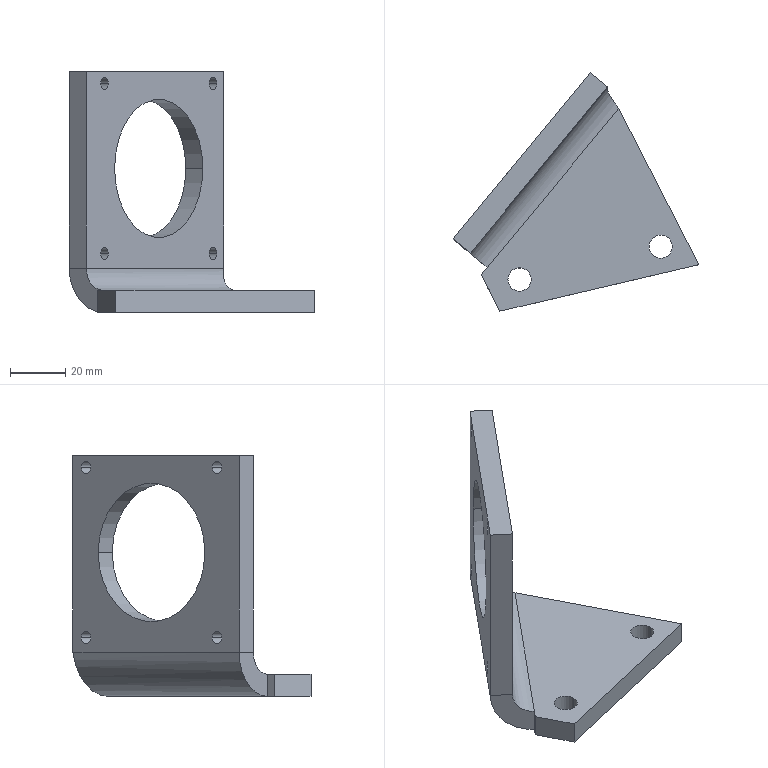Part | SolidWorks | features Cut 2, ICE 2, RefAxis 2, EdgeFlange 1, FlatPattern 1, SMBaseFlange 1, SheetMetal 1 | 1 solid | 29 faces | box 88.743 x 86.001 x 87 mm | volume 61033 mm3 | cylinder 16 | plane 12 | spline 1 | commonest cylinder face diameters 4.4 x8 8.382 x2 8.4 x2 50 x2 16 x1 32 x1
STEP:
#1=CARTESIAN_POINT('',(-8.739,128.402,52.));
#2=VERTEX_POINT('',#1);
#3=CARTESIAN_POINT('',(23.129,166.93,52.));
#4=VERTEX_POINT('',#3);
#5=CARTESIAN_POINT('',(7.195,147.666,52.));
#6=DIRECTION('',(0.7706,-0.6374,0.));
#7=DIRECTION('',(0.6374,0.7706,0.));
#8=AXIS2_PLACEMENT_3D('',#5,#6,#7);
#9=CIRCLE('',#8,25.);
#10=EDGE_CURVE('',#2,#4,#9,.T.);
#11=ORIENTED_EDGE('',*,*,#10,.F.);
#12=CARTESIAN_POINT('',(-2.574,123.303,52.));
#13=VERTEX_POINT('',#12);
#14=CARTESIAN_POINT('',(-10.28,129.677,52.));
#15=DIRECTION('',(0.7706,-0.6374,0.));
#16=VECTOR('',#15,1000.);
#17=LINE('',#14,#16);
#18=EDGE_CURVE('',#2,#13,#17,.T.);
#19=ORIENTED_EDGE('',*,*,#18,.T.);
#20=CARTESIAN_POINT('',(29.293,161.832,52.));
#21=VERTEX_POINT('',#20);
#22=CARTESIAN_POINT('',(13.36,142.567,52.));
#23=DIRECTION('',(0.7706,-0.6374,0.));
#24=DIRECTION('',(0.6374,0.7706,0.));
#25=AXIS2_PLACEMENT_3D('',#22,#23,#24);
#26=CIRCLE('',#25,25.);
#27=EDGE_CURVE('',#13,#21,#26,.T.);
#28=ORIENTED_EDGE('',*,*,#27,.T.);
#29=CARTESIAN_POINT('',(21.588,168.205,52.));
#30=DIRECTION('',(0.7706,-0.6374,0.));
#31=VECTOR('',#30,1000.);
#32=LINE('',#29,#31);
#33=EDGE_CURVE('',#4,#21,#32,.T.);
#34=ORIENTED_EDGE('',*,*,#33,.F.);
#35=EDGE_LOOP('',(#11,#19,#28,#34));
#36=FACE_OUTER_BOUND('',#35,.T.);
#37=CARTESIAN_POINT('',(5.654,148.941,52.));
#38=DIRECTION('',(0.7706,-0.6374,0.));
#39=DIRECTION('',(0.6374,0.7706,0.));
#40=AXIS2_PLACEMENT_3D('',#37,#38,#39);
#41=CYLINDRICAL_SURFACE('',#40,25.);
#42=ADVANCED_FACE('',(#36),#41,.F.);
#43=CARTESIAN_POINT('',(-13.806,122.276,82.75));
#44=VERTEX_POINT('',#43);
#45=CARTESIAN_POINT('',(-11.002,125.666,82.75));
#46=VERTEX_POINT('',#45);
#47=CARTESIAN_POINT('',(-12.404,123.971,82.75));
#48=DIRECTION('',(0.7706,-0.6374,0.));
#49=DIRECTION('',(0.6374,0.7706,0.));
#50=AXIS2_PLACEMENT_3D('',#47,#48,#49);
#51=CIRCLE('',#50,2.2);
#52=EDGE_CURVE('',#44,#46,#51,.T.);
#53=ORIENTED_EDGE('',*,*,#52,.F.);
#54=CARTESIAN_POINT('',(-7.641,117.177,82.75));
#55=VERTEX_POINT('',#54);
#56=CARTESIAN_POINT('',(-15.347,123.551,82.75));
#57=DIRECTION('',(0.7706,-0.6374,0.));
#58=VECTOR('',#57,1000.);
#59=LINE('',#56,#58);
#60=EDGE_CURVE('',#44,#55,#59,.T.);
#61=ORIENTED_EDGE('',*,*,#60,.T.);
#62=CARTESIAN_POINT('',(-4.837,120.568,82.75));
#63=VERTEX_POINT('',#62);
#64=CARTESIAN_POINT('',(-6.239,118.872,82.75));
#65=DIRECTION('',(0.7706,-0.6374,0.));
#66=DIRECTION('',(0.6374,0.7706,0.));
#67=AXIS2_PLACEMENT_3D('',#64,#65,#66);
#68=CIRCLE('',#67,2.2);
#69=EDGE_CURVE('',#55,#63,#68,.T.);
#70=ORIENTED_EDGE('',*,*,#69,.T.);
#71=CARTESIAN_POINT('',(-12.543,126.941,82.75));
#72=DIRECTION('',(0.7706,-0.6374,0.));
#73=VECTOR('',#72,1000.);
#74=LINE('',#71,#73);
#75=EDGE_CURVE('',#46,#63,#74,.T.);
#76=ORIENTED_EDGE('',*,*,#75,.F.);
#77=EDGE_LOOP('',(#53,#61,#70,#76));
#78=FACE_OUTER_BOUND('',#77,.T.);
#79=CARTESIAN_POINT('',(-13.945,125.246,82.75));
#80=DIRECTION('',(0.7706,-0.6374,0.));
#81=DIRECTION('',(0.6374,0.7706,0.));
#82=AXIS2_PLACEMENT_3D('',#79,#80,#81);
#83=CYLINDRICAL_SURFACE('',#82,2.2);
#84=ADVANCED_FACE('',(#78),#83,.F.);
#85=CARTESIAN_POINT('',(-13.806,122.276,21.25));
#86=VERTEX_POINT('',#85);
#87=CARTESIAN_POINT('',(-11.002,125.666,21.25));
#88=VERTEX_POINT('',#87);
#89=CARTESIAN_POINT('',(-12.404,123.971,21.25));
#90=DIRECTION('',(0.7706,-0.6374,0.));
#91=DIRECTION('',(0.6374,0.7706,0.));
#92=AXIS2_PLACEMENT_3D('',#89,#90,#91);
#93=CIRCLE('',#92,2.2);
#94=EDGE_CURVE('',#86,#88,#93,.T.);
#95=ORIENTED_EDGE('',*,*,#94,.F.);
#96=CARTESIAN_POINT('',(-7.641,117.177,21.25));
#97=VERTEX_POINT('',#96);
#98=CARTESIAN_POINT('',(-15.347,123.551,21.25));
#99=DIRECTION('',(0.7706,-0.6374,0.));
#100=VECTOR('',#99,1000.);
#101=LINE('',#98,#100);
#102=EDGE_CURVE('',#86,#97,#101,.T.);
#103=ORIENTED_EDGE('',*,*,#102,.T.);
#104=CARTESIAN_POINT('',(-4.837,120.568,21.25));
#105=VERTEX_POINT('',#104);
#106=CARTESIAN_POINT('',(-6.239,118.872,21.25));
#107=DIRECTION('',(0.7706,-0.6374,0.));
#108=DIRECTION('',(0.6374,0.7706,0.));
#109=AXIS2_PLACEMENT_3D('',#106,#107,#108);
#110=CIRCLE('',#109,2.2);
#111=EDGE_CURVE('',#97,#105,#110,.T.);
#112=ORIENTED_EDGE('',*,*,#111,.T.);
#113=CARTESIAN_POINT('',(-12.543,126.941,21.25));
#114=DIRECTION('',(0.7706,-0.6374,0.));
#115=VECTOR('',#114,1000.);
#116=LINE('',#113,#115);
#117=EDGE_CURVE('',#88,#105,#116,.T.);
#118=ORIENTED_EDGE('',*,*,#117,.F.);
#119=EDGE_LOOP('',(#95,#103,#112,#118));
#120=FACE_OUTER_BOUND('',#119,.T.);
#121=CARTESIAN_POINT('',(-13.945,125.246,21.25));
#122=DIRECTION('',(0.7706,-0.6374,0.));
#123=DIRECTION('',(0.6374,0.7706,0.));
#124=AXIS2_PLACEMENT_3D('',#121,#122,#123);
#125=CYLINDRICAL_SURFACE('',#124,2.2);
#126=ADVANCED_FACE('',(#120),#125,.F.);
#127=CARTESIAN_POINT('',(25.391,169.666,21.25));
#128=VERTEX_POINT('',#127);
#129=CARTESIAN_POINT('',(28.196,173.057,21.25));
#130=VERTEX_POINT('',#129);
#131=CARTESIAN_POINT('',(26.794,171.361,21.25));
#132=DIRECTION('',(0.7706,-0.6374,0.));
#133=DIRECTION('',(0.6374,0.7706,0.));
#134=AXIS2_PLACEMENT_3D('',#131,#132,#133);
#135=CIRCLE('',#134,2.2);
#136=EDGE_CURVE('',#128,#130,#135,.T.);
#137=ORIENTED_EDGE('',*,*,#136,.F.);
#138=CARTESIAN_POINT('',(31.556,164.567,21.25));
#139=VERTEX_POINT('',#138);
#140=CARTESIAN_POINT('',(23.85,170.941,21.25));
#141=DIRECTION('',(0.7706,-0.6374,0.));
#142=VECTOR('',#141,1000.);
#143=LINE('',#140,#142);
#144=EDGE_CURVE('',#128,#139,#143,.T.);
#145=ORIENTED_EDGE('',*,*,#144,.T.);
#146=CARTESIAN_POINT('',(34.36,167.958,21.25));
#147=VERTEX_POINT('',#146);
#148=CARTESIAN_POINT('',(32.958,166.262,21.25));
#149=DIRECTION('',(0.7706,-0.6374,0.));
#150=DIRECTION('',(0.6374,0.7706,0.));
#151=AXIS2_PLACEMENT_3D('',#148,#149,#150);
#152=CIRCLE('',#151,2.2);
#153=EDGE_CURVE('',#139,#147,#152,.T.);
#154=ORIENTED_EDGE('',*,*,#153,.T.);
#155=CARTESIAN_POINT('',(26.655,174.331,21.25));
#156=DIRECTION('',(0.7706,-0.6374,0.));
#157=VECTOR('',#156,1000.);
#158=LINE('',#155,#157);
#159=EDGE_CURVE('',#130,#147,#158,.T.);
#160=ORIENTED_EDGE('',*,*,#159,.F.);
#161=EDGE_LOOP('',(#137,#145,#154,#160));
#162=FACE_OUTER_BOUND('',#161,.T.);
#163=CARTESIAN_POINT('',(25.252,172.636,21.25));
#164=DIRECTION('',(0.7706,-0.6374,0.));
#165=DIRECTION('',(0.6374,0.7706,0.));
#166=AXIS2_PLACEMENT_3D('',#163,#164,#165);
#167=CYLINDRICAL_SURFACE('',#166,2.2);
#168=ADVANCED_FACE('',(#162),#167,.F.);
#169=CARTESIAN_POINT('',(25.391,169.666,82.75));
#170=VERTEX_POINT('',#169);
#171=CARTESIAN_POINT('',(28.196,173.057,82.75));
#172=VERTEX_POINT('',#171);
#173=CARTESIAN_POINT('',(26.794,171.361,82.75));
#174=DIRECTION('',(0.7706,-0.6374,0.));
#175=DIRECTION('',(0.6374,0.7706,0.));
#176=AXIS2_PLACEMENT_3D('',#173,#174,#175);
#177=CIRCLE('',#176,2.2);
#178=EDGE_CURVE('',#170,#172,#177,.T.);
#179=ORIENTED_EDGE('',*,*,#178,.F.);
#180=CARTESIAN_POINT('',(31.556,164.567,82.75));
#181=VERTEX_POINT('',#180);
#182=CARTESIAN_POINT('',(23.85,170.941,82.75));
#183=DIRECTION('',(0.7706,-0.6374,0.));
#184=VECTOR('',#183,1000.);
#185=LINE('',#182,#184);
#186=EDGE_CURVE('',#170,#181,#185,.T.);
#187=ORIENTED_EDGE('',*,*,#186,.T.);
#188=CARTESIAN_POINT('',(34.36,167.958,82.75));
#189=VERTEX_POINT('',#188);
#190=CARTESIAN_POINT('',(32.958,166.262,82.75));
#191=DIRECTION('',(0.7706,-0.6374,0.));
#192=DIRECTION('',(0.6374,0.7706,0.));
#193=AXIS2_PLACEMENT_3D('',#190,#191,#192);
#194=CIRCLE('',#193,2.2);
#195=EDGE_CURVE('',#181,#189,#194,.T.);
#196=ORIENTED_EDGE('',*,*,#195,.T.);
#197=CARTESIAN_POINT('',(26.655,174.331,82.75));
#198=DIRECTION('',(0.7706,-0.6374,0.));
#199=VECTOR('',#198,1000.);
#200=LINE('',#197,#199);
#201=EDGE_CURVE('',#172,#189,#200,.T.);
#202=ORIENTED_EDGE('',*,*,#201,.F.);
#203=EDGE_LOOP('',(#179,#187,#196,#202));
#204=FACE_OUTER_BOUND('',#203,.T.);
#205=CARTESIAN_POINT('',(25.252,172.636,82.75));
#206=DIRECTION('',(0.7706,-0.6374,0.));
#207=DIRECTION('',(0.6374,0.7706,0.));
#208=AXIS2_PLACEMENT_3D('',#205,#206,#207);
#209=CYLINDRICAL_SURFACE('',#208,2.2);
#210=ADVANCED_FACE('',(#204),#209,.F.);
#211=CARTESIAN_POINT('',(51.799,113.384,8.));
#212=VERTEX_POINT('',#211);
#213=CARTESIAN_POINT('',(60.181,113.384,8.));
#214=VERTEX_POINT('',#213);
#215=CARTESIAN_POINT('',(55.99,113.384,8.));
#216=DIRECTION('',(0.,0.,1.));
#217=DIRECTION('',(1.,0.,0.));
#218=AXIS2_PLACEMENT_3D('',#215,#216,#217);
#219=CIRCLE('',#218,4.191);
#220=EDGE_CURVE('',#212,#214,#219,.T.);
#221=ORIENTED_EDGE('',*,*,#220,.T.);
#222=CARTESIAN_POINT('',(60.181,113.384,0.));
#223=VERTEX_POINT('',#222);
#224=CARTESIAN_POINT('',(60.181,113.384,8.));
#225=DIRECTION('',(0.,0.,-1.));
#226=VECTOR('',#225,1000.);
#227=LINE('',#224,#226);
#228=EDGE_CURVE('',#214,#223,#227,.T.);
#229=ORIENTED_EDGE('',*,*,#228,.T.);
#230=CARTESIAN_POINT('',(51.799,113.384,0.));
#231=VERTEX_POINT('',#230);
#232=CARTESIAN_POINT('',(55.99,113.384,0.));
#233=DIRECTION('',(0.,0.,1.));
#234=DIRECTION('',(1.,0.,0.));
#235=AXIS2_PLACEMENT_3D('',#232,#233,#234);
#236=CIRCLE('',#235,4.191);
#237=EDGE_CURVE('',#231,#223,#236,.T.);
#238=ORIENTED_EDGE('',*,*,#237,.F.);
#239=CARTESIAN_POINT('',(51.799,113.384,8.));
#240=DIRECTION('',(0.,0.,-1.));
#241=VECTOR('',#240,1000.);
#242=LINE('',#239,#241);
#243=EDGE_CURVE('',#212,#231,#242,.T.);
#244=ORIENTED_EDGE('',*,*,#243,.F.);
#245=EDGE_LOOP('',(#221,#229,#238,#244));
#246=FACE_OUTER_BOUND('',#245,.T.);
#247=CARTESIAN_POINT('',(55.99,113.384,8.));
#248=DIRECTION('',(0.,0.,-1.));
#249=DIRECTION('',(-1.,0.,0.));
#250=AXIS2_PLACEMENT_3D('',#247,#248,#249);
#251=CYLINDRICAL_SURFACE('',#250,4.191);
#252=ADVANCED_FACE('',(#246),#251,.F.);
#253=CARTESIAN_POINT('',(0.7986,101.477,8.));
#254=VERTEX_POINT('',#253);
#255=CARTESIAN_POINT('',(9.199,101.477,8.));
#256=VERTEX_POINT('',#255);
#257=CARTESIAN_POINT('',(4.999,101.477,8.));
#258=DIRECTION('',(0.,0.,1.));
#259=DIRECTION('',(1.,0.,0.));
#260=AXIS2_PLACEMENT_3D('',#257,#258,#259);
#261=CIRCLE('',#260,4.2);
#262=EDGE_CURVE('',#254,#256,#261,.T.);
#263=ORIENTED_EDGE('',*,*,#262,.T.);
#264=CARTESIAN_POINT('',(9.199,101.477,0.));
#265=VERTEX_POINT('',#264);
#266=CARTESIAN_POINT('',(9.199,101.477,8.));
#267=DIRECTION('',(0.,0.,-1.));
#268=VECTOR('',#267,1000.);
#269=LINE('',#266,#268);
#270=EDGE_CURVE('',#256,#265,#269,.T.);
#271=ORIENTED_EDGE('',*,*,#270,.T.);
#272=CARTESIAN_POINT('',(0.7986,101.477,0.));
#273=VERTEX_POINT('',#272);
#274=CARTESIAN_POINT('',(4.999,101.477,0.));
#275=DIRECTION('',(0.,0.,1.));
#276=DIRECTION('',(1.,0.,0.));
#277=AXIS2_PLACEMENT_3D('',#274,#275,#276);
#278=CIRCLE('',#277,4.2);
#279=EDGE_CURVE('',#273,#265,#278,.T.);
#280=ORIENTED_EDGE('',*,*,#279,.F.);
#281=CARTESIAN_POINT('',(0.7986,101.477,8.));
#282=DIRECTION('',(0.,0.,-1.));
#283=VECTOR('',#282,1000.);
#284=LINE('',#281,#283);
#285=EDGE_CURVE('',#254,#273,#284,.T.);
#286=ORIENTED_EDGE('',*,*,#285,.F.);
#287=EDGE_LOOP('',(#263,#271,#280,#286));
#288=FACE_OUTER_BOUND('',#287,.T.);
#289=CARTESIAN_POINT('',(4.999,101.477,8.));
#290=DIRECTION('',(0.,0.,-1.));
#291=DIRECTION('',(-1.,0.,0.));
#292=AXIS2_PLACEMENT_3D('',#289,#290,#291);
#293=CYLINDRICAL_SURFACE('',#292,4.2);
#294=ADVANCED_FACE('',(#288),#293,.F.);
#295=CARTESIAN_POINT('',(-8.851,103.162,8.));
#296=VERTEX_POINT('',#295);
#297=CARTESIAN_POINT('',(-2.111,90.036,8.));
#298=VERTEX_POINT('',#297);
#299=CARTESIAN_POINT('',(-2.111,90.036,8.));
#300=DIRECTION('',(0.4568,-0.8896,0.));
#301=VECTOR('',#300,1000.);
#302=LINE('',#299,#301);
#303=EDGE_CURVE('',#296,#298,#302,.T.);
#304=ORIENTED_EDGE('',*,*,#303,.T.);
#305=CARTESIAN_POINT('',(69.75,106.816,8.));
#306=VERTEX_POINT('',#305);
#307=CARTESIAN_POINT('',(-2.111,90.036,8.));
#308=DIRECTION('',(0.9738,0.2274,0.));
#309=VECTOR('',#308,1000.);
#310=LINE('',#307,#309);
#311=EDGE_CURVE('',#298,#306,#310,.T.);
#312=ORIENTED_EDGE('',*,*,#311,.T.);
#313=CARTESIAN_POINT('',(40.801,163.193,8.));
#314=VERTEX_POINT('',#313);
#315=CARTESIAN_POINT('',(69.75,106.816,8.));
#316=DIRECTION('',(-0.4568,0.8896,0.));
#317=VECTOR('',#316,1000.);
#318=LINE('',#315,#317);
#319=EDGE_CURVE('',#306,#314,#318,.T.);
#320=ORIENTED_EDGE('',*,*,#319,.T.);
#321=CARTESIAN_POINT('',(-6.663,105.808,8.));
#322=VERTEX_POINT('',#321);
#323=CARTESIAN_POINT('',(-6.663,105.808,8.));
#324=DIRECTION('',(0.6374,0.7706,0.));
#325=VECTOR('',#324,1000.);
#326=LINE('',#323,#325);
#327=EDGE_CURVE('',#322,#314,#326,.T.);
#328=ORIENTED_EDGE('',*,*,#327,.F.);
#329=CARTESIAN_POINT('',(-15.35,95.305,8.));
#330=DIRECTION('',(0.6374,0.7706,0.));
#331=VECTOR('',#330,1000.);
#332=LINE('',#329,#331);
#333=EDGE_CURVE('',#296,#322,#332,.T.);
#334=ORIENTED_EDGE('',*,*,#333,.F.);
#335=EDGE_LOOP('',(#304,#312,#320,#328,#334));
#336=FACE_OUTER_BOUND('',#335,.T.);
#337=ORIENTED_EDGE('',*,*,#262,.F.);
#338=CARTESIAN_POINT('',(4.999,101.477,8.));
#339=DIRECTION('',(0.,0.,1.));
#340=DIRECTION('',(1.,0.,0.));
#341=AXIS2_PLACEMENT_3D('',#338,#339,#340);
#342=CIRCLE('',#341,4.2);
#343=EDGE_CURVE('',#256,#254,#342,.T.);
#344=ORIENTED_EDGE('',*,*,#343,.F.);
#345=EDGE_LOOP('',(#337,#344));
#346=FACE_BOUND('',#345,.T.);
#347=ORIENTED_EDGE('',*,*,#220,.F.);
#348=CARTESIAN_POINT('',(55.99,113.384,8.));
#349=DIRECTION('',(0.,0.,1.));
#350=DIRECTION('',(1.,0.,0.));
#351=AXIS2_PLACEMENT_3D('',#348,#349,#350);
#352=CIRCLE('',#351,4.191);
#353=EDGE_CURVE('',#214,#212,#352,.T.);
#354=ORIENTED_EDGE('',*,*,#353,.F.);
#355=EDGE_LOOP('',(#347,#354));
#356=FACE_BOUND('',#355,.T.);
#357=CARTESIAN_POINT('',(0.,0.,8.));
#358=DIRECTION('',(0.,0.,-1.));
#359=DIRECTION('',(-1.,0.,0.));
#360=AXIS2_PLACEMENT_3D('',#357,#358,#359);
#361=PLANE('',#360);
#362=ADVANCED_FACE('',(#336,#346,#356),#361,.F.);
#363=CARTESIAN_POINT('',(-2.111,90.036,0.));
#364=VERTEX_POINT('',#363);
#365=CARTESIAN_POINT('',(69.75,106.816,0.));
#366=VERTEX_POINT('',#365);
#367=CARTESIAN_POINT('',(-2.111,90.036,0.));
#368=DIRECTION('',(0.9738,0.2274,0.));
#369=VECTOR('',#368,1000.);
#370=LINE('',#367,#369);
#371=EDGE_CURVE('',#364,#366,#370,.T.);
#372=ORIENTED_EDGE('',*,*,#371,.F.);
#373=CARTESIAN_POINT('',(-8.851,103.162,0.));
#374=VERTEX_POINT('',#373);
#375=CARTESIAN_POINT('',(-2.111,90.036,0.));
#376=DIRECTION('',(0.4568,-0.8896,0.));
#377=VECTOR('',#376,1000.);
#378=LINE('',#375,#377);
#379=EDGE_CURVE('',#374,#364,#378,.T.);
#380=ORIENTED_EDGE('',*,*,#379,.F.);
#381=CARTESIAN_POINT('',(-6.663,105.808,0.));
#382=VERTEX_POINT('',#381);
#383=CARTESIAN_POINT('',(-15.35,95.305,0.));
#384=DIRECTION('',(0.6374,0.7706,0.));
#385=VECTOR('',#384,1000.);
#386=LINE('',#383,#385);
#387=EDGE_CURVE('',#374,#382,#386,.T.);
#388=ORIENTED_EDGE('',*,*,#387,.T.);
#389=CARTESIAN_POINT('',(40.801,163.193,0.));
#390=VERTEX_POINT('',#389);
#391=CARTESIAN_POINT('',(-6.663,105.808,0.));
#392=DIRECTION('',(0.6374,0.7706,0.));
#393=VECTOR('',#392,1000.);
#394=LINE('',#391,#393);
#395=EDGE_CURVE('',#382,#390,#394,.T.);
#396=ORIENTED_EDGE('',*,*,#395,.T.);
#397=CARTESIAN_POINT('',(69.75,106.816,0.));
#398=DIRECTION('',(-0.4568,0.8896,0.));
#399=VECTOR('',#398,1000.);
#400=LINE('',#397,#399);
#401=EDGE_CURVE('',#366,#390,#400,.T.);
#402=ORIENTED_EDGE('',*,*,#401,.F.);
#403=EDGE_LOOP('',(#372,#380,#388,#396,#402));
#404=FACE_OUTER_BOUND('',#403,.T.);
#405=ORIENTED_EDGE('',*,*,#279,.T.);
#406=CARTESIAN_POINT('',(4.999,101.477,0.));
#407=DIRECTION('',(0.,0.,1.));
#408=DIRECTION('',(1.,0.,0.));
#409=AXIS2_PLACEMENT_3D('',#406,#407,#408);
#410=CIRCLE('',#409,4.2);
#411=EDGE_CURVE('',#265,#273,#410,.T.);
#412=ORIENTED_EDGE('',*,*,#411,.T.);
#413=EDGE_LOOP('',(#405,#412));
#414=FACE_BOUND('',#413,.T.);
#415=ORIENTED_EDGE('',*,*,#237,.T.);
#416=CARTESIAN_POINT('',(55.99,113.384,0.));
#417=DIRECTION('',(0.,0.,1.));
#418=DIRECTION('',(1.,0.,0.));
#419=AXIS2_PLACEMENT_3D('',#416,#417,#418);
#420=CIRCLE('',#419,4.191);
#421=EDGE_CURVE('',#223,#231,#420,.T.);
#422=ORIENTED_EDGE('',*,*,#421,.T.);
#423=EDGE_LOOP('',(#415,#422));
#424=FACE_BOUND('',#423,.T.);
#425=CARTESIAN_POINT('',(0.,0.,0.));
#426=DIRECTION('',(0.,0.,-1.));
#427=DIRECTION('',(-1.,0.,0.));
#428=AXIS2_PLACEMENT_3D('',#425,#426,#427);
#429=PLANE('',#428);
#430=ADVANCED_FACE('',(#404,#414,#424),#429,.T.);
#431=ORIENTED_EDGE('',*,*,#379,.T.);
#432=CARTESIAN_POINT('',(-2.111,90.036,8.));
#433=DIRECTION('',(0.,0.,-1.));
#434=VECTOR('',#433,1000.);
#435=LINE('',#432,#434);
#436=EDGE_CURVE('',#298,#364,#435,.T.);
#437=ORIENTED_EDGE('',*,*,#436,.F.);
#438=ORIENTED_EDGE('',*,*,#303,.F.);
#439=CARTESIAN_POINT('',(-8.851,103.162,8.));
#440=DIRECTION('',(0.,0.,1.));
#441=VECTOR('',#440,1000.);
#442=LINE('',#439,#441);
#443=EDGE_CURVE('',#374,#296,#442,.T.);
#444=ORIENTED_EDGE('',*,*,#443,.F.);
#445=EDGE_LOOP('',(#431,#437,#438,#444));
#446=FACE_OUTER_BOUND('',#445,.T.);
#447=CARTESIAN_POINT('',(-2.111,90.036,8.));
#448=DIRECTION('',(0.8896,0.4568,0.));
#449=DIRECTION('',(-0.4568,0.8896,0.));
#450=AXIS2_PLACEMENT_3D('',#447,#448,#449);
#451=PLANE('',#450);
#452=ADVANCED_FACE('',(#446),#451,.F.);
#453=CARTESIAN_POINT('',(40.801,163.193,8.));
#454=DIRECTION('',(0.,0.,-1.));
#455=VECTOR('',#454,1000.);
#456=LINE('',#453,#455);
#457=EDGE_CURVE('',#314,#390,#456,.T.);
#458=ORIENTED_EDGE('',*,*,#457,.F.);
#459=ORIENTED_EDGE('',*,*,#319,.F.);
#460=CARTESIAN_POINT('',(69.75,106.816,8.));
#461=DIRECTION('',(0.,0.,-1.));
#462=VECTOR('',#461,1000.);
#463=LINE('',#460,#462);
#464=EDGE_CURVE('',#306,#366,#463,.T.);
#465=ORIENTED_EDGE('',*,*,#464,.T.);
#466=ORIENTED_EDGE('',*,*,#401,.T.);
#467=EDGE_LOOP('',(#458,#459,#465,#466));
#468=FACE_OUTER_BOUND('',#467,.T.);
#469=CARTESIAN_POINT('',(69.75,106.816,8.));
#470=DIRECTION('',(-0.8896,-0.4568,0.));
#471=DIRECTION('',(0.4568,-0.8896,0.));
#472=AXIS2_PLACEMENT_3D('',#469,#470,#471);
#473=PLANE('',#472);
#474=ADVANCED_FACE('',(#468),#473,.F.);
#475=ORIENTED_EDGE('',*,*,#371,.T.);
#476=ORIENTED_EDGE('',*,*,#464,.F.);
#477=ORIENTED_EDGE('',*,*,#311,.F.);
#478=ORIENTED_EDGE('',*,*,#436,.T.);
#479=EDGE_LOOP('',(#475,#476,#477,#478));
#480=FACE_OUTER_BOUND('',#479,.T.);
#481=CARTESIAN_POINT('',(-2.111,90.036,8.));
#482=DIRECTION('',(-0.2274,0.9738,0.));
#483=DIRECTION('',(-0.9738,-0.2274,0.));
#484=AXIS2_PLACEMENT_3D('',#481,#482,#483);
#485=PLANE('',#484);
#486=ADVANCED_FACE('',(#480),#485,.F.);
#487=ORIENTED_EDGE('',*,*,#270,.F.);
#488=ORIENTED_EDGE('',*,*,#343,.T.);
#489=ORIENTED_EDGE('',*,*,#285,.T.);
#490=ORIENTED_EDGE('',*,*,#411,.F.);
#491=EDGE_LOOP('',(#487,#488,#489,#490));
#492=FACE_OUTER_BOUND('',#491,.T.);
#493=CARTESIAN_POINT('',(4.999,101.477,8.));
#494=DIRECTION('',(0.,0.,-1.));
#495=DIRECTION('',(-1.,0.,0.));
#496=AXIS2_PLACEMENT_3D('',#493,#494,#495);
#497=CYLINDRICAL_SURFACE('',#496,4.2);
#498=ADVANCED_FACE('',(#492),#497,.F.);
#499=ORIENTED_EDGE('',*,*,#228,.F.);
#500=ORIENTED_EDGE('',*,*,#353,.T.);
#501=ORIENTED_EDGE('',*,*,#243,.T.);
#502=ORIENTED_EDGE('',*,*,#421,.F.);
#503=EDGE_LOOP('',(#499,#500,#501,#502));
#504=FACE_OUTER_BOUND('',#503,.T.);
#505=CARTESIAN_POINT('',(55.99,113.384,8.));
#506=DIRECTION('',(0.,0.,-1.));
#507=DIRECTION('',(-1.,0.,0.));
#508=AXIS2_PLACEMENT_3D('',#505,#506,#507);
#509=CYLINDRICAL_SURFACE('',#508,4.191);
#510=ADVANCED_FACE('',(#504),#509,.F.);
#511=CARTESIAN_POINT('',(36.825,170.937,16.));
#512=VERTEX_POINT('',#511);
#513=CARTESIAN_POINT('',(30.66,176.036,16.));
#514=VERTEX_POINT('',#513);
#515=CARTESIAN_POINT('',(36.825,170.937,16.));
#516=DIRECTION('',(-0.7706,0.6374,0.));
#517=VECTOR('',#516,1000.);
#518=LINE('',#515,#517);
#519=EDGE_CURVE('',#512,#514,#518,.T.);
#520=ORIENTED_EDGE('',*,*,#519,.F.);
#521=CARTESIAN_POINT('',(40.801,163.193,8.));
#522=CARTESIAN_POINT('',(40.486,163.641,8.));
#523=CARTESIAN_POINT('',(40.176,164.082,8.052));
#524=CARTESIAN_POINT('',(39.722,164.734,8.204));
#525=CARTESIAN_POINT('',(39.572,164.951,8.267));
#526=CARTESIAN_POINT('',(39.277,165.381,8.419));
#527=CARTESIAN_POINT('',(39.131,165.596,8.508));
#528=CARTESIAN_POINT('',(38.707,166.225,8.81));
#529=CARTESIAN_POINT('',(38.443,166.627,9.055));
#530=CARTESIAN_POINT('',(37.956,167.4,9.635));
#531=CARTESIAN_POINT('',(37.731,167.774,9.972));
#532=CARTESIAN_POINT('',(37.344,168.465,10.711));
#533=CARTESIAN_POINT('',(37.179,168.785,11.113));
#534=CARTESIAN_POINT('',(36.979,169.229,11.766));
#535=CARTESIAN_POINT('',(36.92,169.372,11.993));
#536=CARTESIAN_POINT('',(36.82,169.64,12.456));
#537=CARTESIAN_POINT('',(36.779,169.767,12.692));
#538=CARTESIAN_POINT('',(36.685,170.122,13.415));
#539=CARTESIAN_POINT('',(36.658,170.329,13.913));
#540=CARTESIAN_POINT('',(36.676,170.594,14.687));
#541=CARTESIAN_POINT('',(36.692,170.674,14.949));
#542=CARTESIAN_POINT('',(36.743,170.818,15.473));
#543=CARTESIAN_POINT('',(36.779,170.882,15.736));
#544=CARTESIAN_POINT('',(36.825,170.937,16.));
#545=B_SPLINE_CURVE_WITH_KNOTS('',3,(#521,#522,#523,#524,#525,#526,#527,#528,#529,#530,#531,#532,#533,#534,#535,#536,#537,#538,#539,#540,#541,#542,#543,#544),.UNSPECIFIED.,.F.,.F.,(4,2,2,2,2,2,2,2,2,2,2,4),(0.,0.001619,0.002429,0.003239,0.004858,0.006477,0.008097,0.008906,0.009716,0.01134,0.01215,0.01295),.UNSPECIFIED.);
#546=EDGE_CURVE('',#314,#512,#545,.T.);
#547=ORIENTED_EDGE('',*,*,#546,.F.);
#548=ORIENTED_EDGE('',*,*,#457,.T.);
#549=CARTESIAN_POINT('',(40.801,163.193,0.));
#550=CARTESIAN_POINT('',(40.079,163.978,0.));
#551=CARTESIAN_POINT('',(39.369,164.749,0.1036));
#552=CARTESIAN_POINT('',(38.324,165.891,0.4081));
#553=CARTESIAN_POINT('',(37.979,166.268,0.5345));
#554=CARTESIAN_POINT('',(37.297,167.019,0.8386));
#555=CARTESIAN_POINT('',(36.958,167.393,1.017));
#556=CARTESIAN_POINT('',(35.975,168.485,1.619));
#557=CARTESIAN_POINT('',(35.358,169.179,2.11));
#558=CARTESIAN_POINT('',(34.49,170.175,2.98));
#559=CARTESIAN_POINT('',(34.21,170.499,3.292));
#560=CARTESIAN_POINT('',(33.673,171.131,3.961));
#561=CARTESIAN_POINT('',(33.419,171.433,4.313));
#562=CARTESIAN_POINT('',(32.702,172.304,5.42));
#563=CARTESIAN_POINT('',(32.282,172.835,6.225));
#564=CARTESIAN_POINT('',(31.744,173.559,7.533));
#565=CARTESIAN_POINT('',(31.58,173.789,7.988));
#566=CARTESIAN_POINT('',(31.29,174.215,8.912));
#567=CARTESIAN_POINT('',(31.163,174.412,9.383));
#568=CARTESIAN_POINT('',(30.946,174.776,10.345));
#569=CARTESIAN_POINT('',(30.856,174.943,10.836));
#570=CARTESIAN_POINT('',(30.712,175.247,11.835));
#571=CARTESIAN_POINT('',(30.659,175.384,12.346));
#572=CARTESIAN_POINT('',(30.557,175.749,13.898));
#573=CARTESIAN_POINT('',(30.568,175.925,14.944));
#574=CARTESIAN_POINT('',(30.66,176.036,16.));
#575=B_SPLINE_CURVE_WITH_KNOTS('',3,(#549,#550,#551,#552,#553,#554,#555,#556,#557,#558,#559,#560,#561,#562,#563,#564,#565,#566,#567,#568,#569,#570,#571,#572,#573,#574),.UNSPECIFIED.,.F.,.F.,(4,2,2,2,2,2,2,2,2,2,2,2,4),(0.,0.003153,0.00473,0.006307,0.00946,0.01104,0.01261,0.01577,0.01734,0.01892,0.0205,0.02207,0.02523),.UNSPECIFIED.);
#576=EDGE_CURVE('',#390,#514,#575,.T.);
#577=ORIENTED_EDGE('',*,*,#576,.T.);
#578=EDGE_LOOP('',(#520,#547,#548,#577));
#579=FACE_OUTER_BOUND('',#578,.T.);
#580=CARTESIAN_POINT('',(40.801,163.193,-0.08));
#581=CARTESIAN_POINT('',(39.362,164.755,-0.08));
#582=CARTESIAN_POINT('',(37.923,166.317,0.3385));
#583=CARTESIAN_POINT('',(35.291,169.236,1.95));
#584=CARTESIAN_POINT('',(34.098,170.594,3.141));
#585=CARTESIAN_POINT('',(32.169,172.932,6.118));
#586=CARTESIAN_POINT('',(31.433,173.912,7.902));
#587=CARTESIAN_POINT('',(30.557,175.38,11.791));
#588=CARTESIAN_POINT('',(30.416,175.867,13.895));
#589=CARTESIAN_POINT('',(30.599,176.087,16.));
#590=CARTESIAN_POINT('',(40.801,163.193,0.));
#591=CARTESIAN_POINT('',(39.37,164.749,0.));
#592=CARTESIAN_POINT('',(37.939,166.303,0.4164));
#593=CARTESIAN_POINT('',(35.322,169.211,2.019));
#594=CARTESIAN_POINT('',(34.136,170.562,3.205));
#595=CARTESIAN_POINT('',(32.219,172.891,6.167));
#596=CARTESIAN_POINT('',(31.487,173.867,7.942));
#597=CARTESIAN_POINT('',(30.617,175.33,11.812));
#598=CARTESIAN_POINT('',(30.478,175.816,13.905));
#599=CARTESIAN_POINT('',(30.66,176.036,16.));
#600=CARTESIAN_POINT('',(40.801,163.193,8.));
#601=CARTESIAN_POINT('',(40.177,164.081,8.));
#602=CARTESIAN_POINT('',(39.553,164.969,8.208));
#603=CARTESIAN_POINT('',(38.426,166.643,9.01));
#604=CARTESIAN_POINT('',(37.925,167.429,9.603));
#605=CARTESIAN_POINT('',(37.148,168.814,11.084));
#606=CARTESIAN_POINT('',(36.874,169.412,11.971));
#607=CARTESIAN_POINT('',(36.621,170.364,13.906));
#608=CARTESIAN_POINT('',(36.643,170.717,14.953));
#609=CARTESIAN_POINT('',(36.825,170.937,16.));
#610=CARTESIAN_POINT('',(40.801,163.193,8.081));
#611=CARTESIAN_POINT('',(40.185,164.074,8.081));
#612=CARTESIAN_POINT('',(39.569,164.955,8.287));
#613=CARTESIAN_POINT('',(38.458,166.617,9.08));
#614=CARTESIAN_POINT('',(37.963,167.397,9.667));
#615=CARTESIAN_POINT('',(37.198,168.772,11.133));
#616=CARTESIAN_POINT('',(36.928,169.367,12.012));
#617=CARTESIAN_POINT('',(36.681,170.314,13.927));
#618=CARTESIAN_POINT('',(36.705,170.665,14.963));
#619=CARTESIAN_POINT('',(36.887,170.886,16.));
#620=B_SPLINE_SURFACE_WITH_KNOTS('',1,3,((#580,#581,#582,#583,#584,#585,#586,#587,#588,#589),(#590,#591,#592,#593,#594,#595,#596,#597,#598,#599),(#600,#601,#602,#603,#604,#605,#606,#607,#608,#609),(#610,#611,#612,#613,#614,#615,#616,#617,#618,#619)),.UNSPECIFIED.,.F.,.F.,.F.,(2,1,1,2),(4,2,2,2,4),(-0.01,0.,1.,1.01),(0.,0.25,0.5,0.75,1.),.UNSPECIFIED.);
#621=ADVANCED_FACE('',(#579),#620,.F.);
#622=CARTESIAN_POINT('',(-12.828,110.906,16.));
#623=VERTEX_POINT('',#622);
#624=CARTESIAN_POINT('',(-6.663,105.808,16.));
#625=DIRECTION('',(-0.6374,-0.7706,0.));
#626=DIRECTION('',(0.7706,-0.6374,0.));
#627=AXIS2_PLACEMENT_3D('',#624,#625,#626);
#628=CIRCLE('',#627,8.);
#629=EDGE_CURVE('',#623,#322,#628,.T.);
#630=ORIENTED_EDGE('',*,*,#629,.F.);
#631=CARTESIAN_POINT('',(-18.993,116.005,16.));
#632=VERTEX_POINT('',#631);
#633=CARTESIAN_POINT('',(-12.828,110.906,16.));
#634=DIRECTION('',(-0.7706,0.6374,0.));
#635=VECTOR('',#634,1000.);
#636=LINE('',#633,#635);
#637=EDGE_CURVE('',#623,#632,#636,.T.);
#638=ORIENTED_EDGE('',*,*,#637,.T.);
#639=CARTESIAN_POINT('',(-6.663,105.808,16.));
#640=DIRECTION('',(-0.6374,-0.7706,0.));
#641=DIRECTION('',(0.7706,-0.6374,0.));
#642=AXIS2_PLACEMENT_3D('',#639,#640,#641);
#643=CIRCLE('',#642,16.);
#644=EDGE_CURVE('',#632,#382,#643,.T.);
#645=ORIENTED_EDGE('',*,*,#644,.T.);
#646=CARTESIAN_POINT('',(-6.663,105.808,8.));
#647=DIRECTION('',(0.,0.,-1.));
#648=VECTOR('',#647,1000.);
#649=LINE('',#646,#648);
#650=EDGE_CURVE('',#322,#382,#649,.T.);
#651=ORIENTED_EDGE('',*,*,#650,.F.);
#652=EDGE_LOOP('',(#630,#638,#645,#651));
#653=FACE_OUTER_BOUND('',#652,.T.);
#654=CARTESIAN_POINT('',(-6.663,105.808,16.));
#655=DIRECTION('',(0.6374,0.7706,0.));
#656=DIRECTION('',(-0.7706,0.6374,0.));
#657=AXIS2_PLACEMENT_3D('',#654,#655,#656);
#658=PLANE('',#657);
#659=ADVANCED_FACE('',(#653),#658,.F.);
#660=ORIENTED_EDGE('',*,*,#395,.F.);
#661=ORIENTED_EDGE('',*,*,#644,.F.);
#662=CARTESIAN_POINT('',(-68.251,56.452,16.));
#663=DIRECTION('',(0.6374,0.7706,0.));
#664=VECTOR('',#663,1000.);
#665=LINE('',#662,#664);
#666=EDGE_CURVE('',#632,#514,#665,.T.);
#667=ORIENTED_EDGE('',*,*,#666,.T.);
#668=ORIENTED_EDGE('',*,*,#576,.F.);
#669=EDGE_LOOP('',(#660,#661,#667,#668));
#670=FACE_OUTER_BOUND('',#669,.T.);
#671=CARTESIAN_POINT('',(-6.663,105.808,16.));
#672=DIRECTION('',(-0.6374,-0.7706,0.));
#673=DIRECTION('',(-0.7706,0.6374,0.));
#674=AXIS2_PLACEMENT_3D('',#671,#672,#673);
#675=CYLINDRICAL_SURFACE('',#674,16.);
#676=ADVANCED_FACE('',(#670),#675,.T.);
#677=ORIENTED_EDGE('',*,*,#327,.T.);
#678=ORIENTED_EDGE('',*,*,#546,.T.);
#679=CARTESIAN_POINT('',(36.825,170.937,16.));
#680=DIRECTION('',(-0.6374,-0.7706,0.));
#681=VECTOR('',#680,1000.);
#682=LINE('',#679,#681);
#683=EDGE_CURVE('',#512,#623,#682,.T.);
#684=ORIENTED_EDGE('',*,*,#683,.T.);
#685=ORIENTED_EDGE('',*,*,#629,.T.);
#686=EDGE_LOOP('',(#677,#678,#684,#685));
#687=FACE_OUTER_BOUND('',#686,.T.);
#688=CARTESIAN_POINT('',(-6.663,105.808,16.));
#689=DIRECTION('',(-0.6374,-0.7706,0.));
#690=DIRECTION('',(-0.7706,0.6374,0.));
#691=AXIS2_PLACEMENT_3D('',#688,#689,#690);
#692=CYLINDRICAL_SURFACE('',#691,8.);
#693=ADVANCED_FACE('',(#687),#692,.F.);
#694=ORIENTED_EDGE('',*,*,#519,.T.);
#695=CARTESIAN_POINT('',(30.66,176.036,87.));
#696=VERTEX_POINT('',#695);
#697=CARTESIAN_POINT('',(30.66,176.036,8.));
#698=DIRECTION('',(0.,0.,-1.));
#699=VECTOR('',#698,1000.);
#700=LINE('',#697,#699);
#701=EDGE_CURVE('',#696,#514,#700,.T.);
#702=ORIENTED_EDGE('',*,*,#701,.F.);
#703=CARTESIAN_POINT('',(36.825,170.937,87.));
#704=VERTEX_POINT('',#703);
#705=CARTESIAN_POINT('',(36.825,170.937,87.));
#706=DIRECTION('',(-0.7706,0.6374,0.));
#707=VECTOR('',#706,1000.);
#708=LINE('',#705,#707);
#709=EDGE_CURVE('',#704,#696,#708,.T.);
#710=ORIENTED_EDGE('',*,*,#709,.F.);
#711=CARTESIAN_POINT('',(36.825,170.937,8.));
#712=DIRECTION('',(0.,0.,-1.));
#713=VECTOR('',#712,1000.);
#714=LINE('',#711,#713);
#715=EDGE_CURVE('',#704,#512,#714,.T.);
#716=ORIENTED_EDGE('',*,*,#715,.T.);
#717=EDGE_LOOP('',(#694,#702,#710,#716));
#718=FACE_OUTER_BOUND('',#717,.T.);
#719=CARTESIAN_POINT('',(30.66,176.036,8.));
#720=DIRECTION('',(-0.6374,-0.7706,0.));
#721=DIRECTION('',(0.7706,-0.6374,0.));
#722=AXIS2_PLACEMENT_3D('',#719,#720,#721);
#723=PLANE('',#722);
#724=ADVANCED_FACE('',(#718),#723,.F.);
#725=ORIENTED_EDGE('',*,*,#637,.F.);
#726=CARTESIAN_POINT('',(-12.828,110.906,87.));
#727=VERTEX_POINT('',#726);
#728=CARTESIAN_POINT('',(-12.828,110.906,85.));
#729=DIRECTION('',(0.,0.,1.));
#730=VECTOR('',#729,1000.);
#731=LINE('',#728,#730);
#732=EDGE_CURVE('',#623,#727,#731,.T.);
#733=ORIENTED_EDGE('',*,*,#732,.T.);
#734=CARTESIAN_POINT('',(-18.993,116.005,87.));
#735=VERTEX_POINT('',#734);
#736=CARTESIAN_POINT('',(-18.993,116.005,87.));
#737=DIRECTION('',(0.7706,-0.6374,0.));
#738=VECTOR('',#737,1000.);
#739=LINE('',#736,#738);
#740=EDGE_CURVE('',#735,#727,#739,.T.);
#741=ORIENTED_EDGE('',*,*,#740,.F.);
#742=CARTESIAN_POINT('',(-18.993,116.005,85.));
#743=DIRECTION('',(0.,0.,1.));
#744=VECTOR('',#743,1000.);
#745=LINE('',#742,#744);
#746=EDGE_CURVE('',#632,#735,#745,.T.);
#747=ORIENTED_EDGE('',*,*,#746,.F.);
#748=EDGE_LOOP('',(#725,#733,#741,#747));
#749=FACE_OUTER_BOUND('',#748,.T.);
#750=CARTESIAN_POINT('',(-18.993,116.005,85.));
#751=DIRECTION('',(0.6374,0.7706,0.));
#752=DIRECTION('',(-0.7706,0.6374,0.));
#753=AXIS2_PLACEMENT_3D('',#750,#751,#752);
#754=PLANE('',#753);
#755=ADVANCED_FACE('',(#749),#754,.F.);
#756=CARTESIAN_POINT('',(7.195,147.666,52.));
#757=DIRECTION('',(0.7706,-0.6374,0.));
#758=DIRECTION('',(0.6374,0.7706,0.));
#759=AXIS2_PLACEMENT_3D('',#756,#757,#758);
#760=CIRCLE('',#759,25.);
#761=EDGE_CURVE('',#4,#2,#760,.T.);
#762=ORIENTED_EDGE('',*,*,#761,.T.);
#763=ORIENTED_EDGE('',*,*,#10,.T.);
#764=EDGE_LOOP('',(#762,#763));
#765=FACE_BOUND('',#764,.T.);
#766=CARTESIAN_POINT('',(-12.404,123.971,82.75));
#767=DIRECTION('',(0.7706,-0.6374,0.));
#768=DIRECTION('',(0.6374,0.7706,0.));
#769=AXIS2_PLACEMENT_3D('',#766,#767,#768);
#770=CIRCLE('',#769,2.2);
#771=EDGE_CURVE('',#46,#44,#770,.T.);
#772=ORIENTED_EDGE('',*,*,#771,.T.);
#773=ORIENTED_EDGE('',*,*,#52,.T.);
#774=EDGE_LOOP('',(#772,#773));
#775=FACE_BOUND('',#774,.T.);
#776=CARTESIAN_POINT('',(-12.404,123.971,21.25));
#777=DIRECTION('',(0.7706,-0.6374,0.));
#778=DIRECTION('',(0.6374,0.7706,0.));
#779=AXIS2_PLACEMENT_3D('',#776,#777,#778);
#780=CIRCLE('',#779,2.2);
#781=EDGE_CURVE('',#88,#86,#780,.T.);
#782=ORIENTED_EDGE('',*,*,#781,.T.);
#783=ORIENTED_EDGE('',*,*,#94,.T.);
#784=EDGE_LOOP('',(#782,#783));
#785=FACE_BOUND('',#784,.T.);
#786=CARTESIAN_POINT('',(26.794,171.361,21.25));
#787=DIRECTION('',(0.7706,-0.6374,0.));
#788=DIRECTION('',(0.6374,0.7706,0.));
#789=AXIS2_PLACEMENT_3D('',#786,#787,#788);
#790=CIRCLE('',#789,2.2);
#791=EDGE_CURVE('',#130,#128,#790,.T.);
#792=ORIENTED_EDGE('',*,*,#791,.T.);
#793=ORIENTED_EDGE('',*,*,#136,.T.);
#794=EDGE_LOOP('',(#792,#793));
#795=FACE_BOUND('',#794,.T.);
#796=CARTESIAN_POINT('',(26.794,171.361,82.75));
#797=DIRECTION('',(0.7706,-0.6374,0.));
#798=DIRECTION('',(0.6374,0.7706,0.));
#799=AXIS2_PLACEMENT_3D('',#796,#797,#798);
#800=CIRCLE('',#799,2.2);
#801=EDGE_CURVE('',#172,#170,#800,.T.);
#802=ORIENTED_EDGE('',*,*,#801,.T.);
#803=ORIENTED_EDGE('',*,*,#178,.T.);
#804=EDGE_LOOP('',(#802,#803));
#805=FACE_BOUND('',#804,.T.);
#806=ORIENTED_EDGE('',*,*,#666,.F.);
#807=ORIENTED_EDGE('',*,*,#746,.T.);
#808=CARTESIAN_POINT('',(30.66,176.036,87.));
#809=DIRECTION('',(-0.6374,-0.7706,0.));
#810=VECTOR('',#809,1000.);
#811=LINE('',#808,#810);
#812=EDGE_CURVE('',#696,#735,#811,.T.);
#813=ORIENTED_EDGE('',*,*,#812,.F.);
#814=ORIENTED_EDGE('',*,*,#701,.T.);
#815=EDGE_LOOP('',(#806,#807,#813,#814));
#816=FACE_OUTER_BOUND('',#815,.T.);
#817=CARTESIAN_POINT('',(-68.251,56.452,0.));
#818=DIRECTION('',(0.7706,-0.6374,0.));
#819=DIRECTION('',(0.6374,0.7706,0.));
#820=AXIS2_PLACEMENT_3D('',#817,#818,#819);
#821=PLANE('',#820);
#822=ADVANCED_FACE('',(#765,#775,#785,#795,#805,#816),#821,.F.);
#823=CARTESIAN_POINT('',(13.36,142.567,52.));
#824=DIRECTION('',(0.7706,-0.6374,0.));
#825=DIRECTION('',(0.6374,0.7706,0.));
#826=AXIS2_PLACEMENT_3D('',#823,#824,#825);
#827=CIRCLE('',#826,25.);
#828=EDGE_CURVE('',#21,#13,#827,.T.);
#829=ORIENTED_EDGE('',*,*,#828,.F.);
#830=ORIENTED_EDGE('',*,*,#27,.F.);
#831=EDGE_LOOP('',(#829,#830));
#832=FACE_BOUND('',#831,.T.);
#833=CARTESIAN_POINT('',(-6.239,118.872,82.75));
#834=DIRECTION('',(0.7706,-0.6374,0.));
#835=DIRECTION('',(0.6374,0.7706,0.));
#836=AXIS2_PLACEMENT_3D('',#833,#834,#835);
#837=CIRCLE('',#836,2.2);
#838=EDGE_CURVE('',#63,#55,#837,.T.);
#839=ORIENTED_EDGE('',*,*,#838,.F.);
#840=ORIENTED_EDGE('',*,*,#69,.F.);
#841=EDGE_LOOP('',(#839,#840));
#842=FACE_BOUND('',#841,.T.);
#843=CARTESIAN_POINT('',(-6.239,118.872,21.25));
#844=DIRECTION('',(0.7706,-0.6374,0.));
#845=DIRECTION('',(0.6374,0.7706,0.));
#846=AXIS2_PLACEMENT_3D('',#843,#844,#845);
#847=CIRCLE('',#846,2.2);
#848=EDGE_CURVE('',#105,#97,#847,.T.);
#849=ORIENTED_EDGE('',*,*,#848,.F.);
#850=ORIENTED_EDGE('',*,*,#111,.F.);
#851=EDGE_LOOP('',(#849,#850));
#852=FACE_BOUND('',#851,.T.);
#853=CARTESIAN_POINT('',(32.958,166.262,21.25));
#854=DIRECTION('',(0.7706,-0.6374,0.));
#855=DIRECTION('',(0.6374,0.7706,0.));
#856=AXIS2_PLACEMENT_3D('',#853,#854,#855);
#857=CIRCLE('',#856,2.2);
#858=EDGE_CURVE('',#147,#139,#857,.T.);
#859=ORIENTED_EDGE('',*,*,#858,.F.);
#860=ORIENTED_EDGE('',*,*,#153,.F.);
#861=EDGE_LOOP('',(#859,#860));
#862=FACE_BOUND('',#861,.T.);
#863=CARTESIAN_POINT('',(32.958,166.262,82.75));
#864=DIRECTION('',(0.7706,-0.6374,0.));
#865=DIRECTION('',(0.6374,0.7706,0.));
#866=AXIS2_PLACEMENT_3D('',#863,#864,#865);
#867=CIRCLE('',#866,2.2);
#868=EDGE_CURVE('',#189,#181,#867,.T.);
#869=ORIENTED_EDGE('',*,*,#868,.F.);
#870=ORIENTED_EDGE('',*,*,#195,.F.);
#871=EDGE_LOOP('',(#869,#870));
#872=FACE_BOUND('',#871,.T.);
#873=ORIENTED_EDGE('',*,*,#732,.F.);
#874=ORIENTED_EDGE('',*,*,#683,.F.);
#875=ORIENTED_EDGE('',*,*,#715,.F.);
#876=CARTESIAN_POINT('',(-12.828,110.906,87.));
#877=DIRECTION('',(0.6374,0.7706,0.));
#878=VECTOR('',#877,1000.);
#879=LINE('',#876,#878);
#880=EDGE_CURVE('',#727,#704,#879,.T.);
#881=ORIENTED_EDGE('',*,*,#880,.F.);
#882=EDGE_LOOP('',(#873,#874,#875,#881));
#883=FACE_OUTER_BOUND('',#882,.T.);
#884=CARTESIAN_POINT('',(-62.086,51.353,0.));
#885=DIRECTION('',(0.7706,-0.6374,0.));
#886=DIRECTION('',(0.6374,0.7706,0.));
#887=AXIS2_PLACEMENT_3D('',#884,#885,#886);
#888=PLANE('',#887);
#889=ADVANCED_FACE('',(#832,#842,#852,#862,#872,#883),#888,.T.);
#890=ORIENTED_EDGE('',*,*,#186,.F.);
#891=ORIENTED_EDGE('',*,*,#801,.F.);
#892=ORIENTED_EDGE('',*,*,#201,.T.);
#893=ORIENTED_EDGE('',*,*,#868,.T.);
#894=EDGE_LOOP('',(#890,#891,#892,#893));
#895=FACE_OUTER_BOUND('',#894,.T.);
#896=CARTESIAN_POINT('',(25.252,172.636,82.75));
#897=DIRECTION('',(0.7706,-0.6374,0.));
#898=DIRECTION('',(0.6374,0.7706,0.));
#899=AXIS2_PLACEMENT_3D('',#896,#897,#898);
#900=CYLINDRICAL_SURFACE('',#899,2.2);
#901=ADVANCED_FACE('',(#895),#900,.F.);
#902=ORIENTED_EDGE('',*,*,#144,.F.);
#903=ORIENTED_EDGE('',*,*,#791,.F.);
#904=ORIENTED_EDGE('',*,*,#159,.T.);
#905=ORIENTED_EDGE('',*,*,#858,.T.);
#906=EDGE_LOOP('',(#902,#903,#904,#905));
#907=FACE_OUTER_BOUND('',#906,.T.);
#908=CARTESIAN_POINT('',(25.252,172.636,21.25));
#909=DIRECTION('',(0.7706,-0.6374,0.));
#910=DIRECTION('',(0.6374,0.7706,0.));
#911=AXIS2_PLACEMENT_3D('',#908,#909,#910);
#912=CYLINDRICAL_SURFACE('',#911,2.2);
#913=ADVANCED_FACE('',(#907),#912,.F.);
#914=ORIENTED_EDGE('',*,*,#102,.F.);
#915=ORIENTED_EDGE('',*,*,#781,.F.);
#916=ORIENTED_EDGE('',*,*,#117,.T.);
#917=ORIENTED_EDGE('',*,*,#848,.T.);
#918=EDGE_LOOP('',(#914,#915,#916,#917));
#919=FACE_OUTER_BOUND('',#918,.T.);
#920=CARTESIAN_POINT('',(-13.945,125.246,21.25));
#921=DIRECTION('',(0.7706,-0.6374,0.));
#922=DIRECTION('',(0.6374,0.7706,0.));
#923=AXIS2_PLACEMENT_3D('',#920,#921,#922);
#924=CYLINDRICAL_SURFACE('',#923,2.2);
#925=ADVANCED_FACE('',(#919),#924,.F.);
#926=ORIENTED_EDGE('',*,*,#60,.F.);
#927=ORIENTED_EDGE('',*,*,#771,.F.);
#928=ORIENTED_EDGE('',*,*,#75,.T.);
#929=ORIENTED_EDGE('',*,*,#838,.T.);
#930=EDGE_LOOP('',(#926,#927,#928,#929));
#931=FACE_OUTER_BOUND('',#930,.T.);
#932=CARTESIAN_POINT('',(-13.945,125.246,82.75));
#933=DIRECTION('',(0.7706,-0.6374,0.));
#934=DIRECTION('',(0.6374,0.7706,0.));
#935=AXIS2_PLACEMENT_3D('',#932,#933,#934);
#936=CYLINDRICAL_SURFACE('',#935,2.2);
#937=ADVANCED_FACE('',(#931),#936,.F.);
#938=ORIENTED_EDGE('',*,*,#18,.F.);
#939=ORIENTED_EDGE('',*,*,#761,.F.);
#940=ORIENTED_EDGE('',*,*,#33,.T.);
#941=ORIENTED_EDGE('',*,*,#828,.T.);
#942=EDGE_LOOP('',(#938,#939,#940,#941));
#943=FACE_OUTER_BOUND('',#942,.T.);
#944=CARTESIAN_POINT('',(5.654,148.941,52.));
#945=DIRECTION('',(0.7706,-0.6374,0.));
#946=DIRECTION('',(0.6374,0.7706,0.));
#947=AXIS2_PLACEMENT_3D('',#944,#945,#946);
#948=CYLINDRICAL_SURFACE('',#947,25.);
#949=ADVANCED_FACE('',(#943),#948,.F.);
#950=ORIENTED_EDGE('',*,*,#812,.T.);
#951=ORIENTED_EDGE('',*,*,#740,.T.);
#952=ORIENTED_EDGE('',*,*,#880,.T.);
#953=ORIENTED_EDGE('',*,*,#709,.T.);
#954=EDGE_LOOP('',(#950,#951,#952,#953));
#955=FACE_OUTER_BOUND('',#954,.T.);
#956=CARTESIAN_POINT('',(12.138,143.577,87.));
#957=DIRECTION('',(0.,0.,1.));
#958=DIRECTION('',(-0.7706,0.6374,0.));
#959=AXIS2_PLACEMENT_3D('',#956,#957,#958);
#960=PLANE('',#959);
#961=ADVANCED_FACE('',(#955),#960,.T.);
#962=ORIENTED_EDGE('',*,*,#387,.F.);
#963=ORIENTED_EDGE('',*,*,#443,.T.);
#964=ORIENTED_EDGE('',*,*,#333,.T.);
#965=ORIENTED_EDGE('',*,*,#650,.T.);
#966=EDGE_LOOP('',(#962,#963,#964,#965));
#967=FACE_OUTER_BOUND('',#966,.T.);
#968=CARTESIAN_POINT('',(-15.35,95.305,8.));
#969=DIRECTION('',(0.7706,-0.6374,0.));
#970=DIRECTION('',(0.6374,0.7706,0.));
#971=AXIS2_PLACEMENT_3D('',#968,#969,#970);
#972=PLANE('',#971);
#973=ADVANCED_FACE('',(#967),#972,.F.);
#974=CLOSED_SHELL('',(#42,#84,#126,#168,#210,#252,#294,#362,#430,#452,#474,#486,#498,#510,#621,#659,#676,#693,#724,#755,#822,#889,#901,#913,#925,#937,#949,#961,#973));
#975=MANIFOLD_SOLID_BREP('',#974);
#976=CARTESIAN_POINT('',(0.,0.,0.));
#977=DIRECTION('',(0.,0.,1.));
#978=DIRECTION('',(1.,0.,0.));
#979=AXIS2_PLACEMENT_3D('',#976,#977,#978);
#980=(LENGTH_UNIT()NAMED_UNIT(*)SI_UNIT(.MILLI.,.METRE.));
#981=UNCERTAINTY_MEASURE_WITH_UNIT(LENGTH_MEASURE(0.00001),#980,'','');
#982=(NAMED_UNIT(*)PLANE_ANGLE_UNIT()SI_UNIT($,.RADIAN.));
#983=(NAMED_UNIT(*)SI_UNIT($,.STERADIAN.)SOLID_ANGLE_UNIT());
#984=(GEOMETRIC_REPRESENTATION_CONTEXT(3)GLOBAL_UNCERTAINTY_ASSIGNED_CONTEXT((#981))GLOBAL_UNIT_ASSIGNED_CONTEXT((#980,#982,#983))REPRESENTATION_CONTEXT('',''));
#985=ADVANCED_BREP_SHAPE_REPRESENTATION('',(#975,#979),#984);